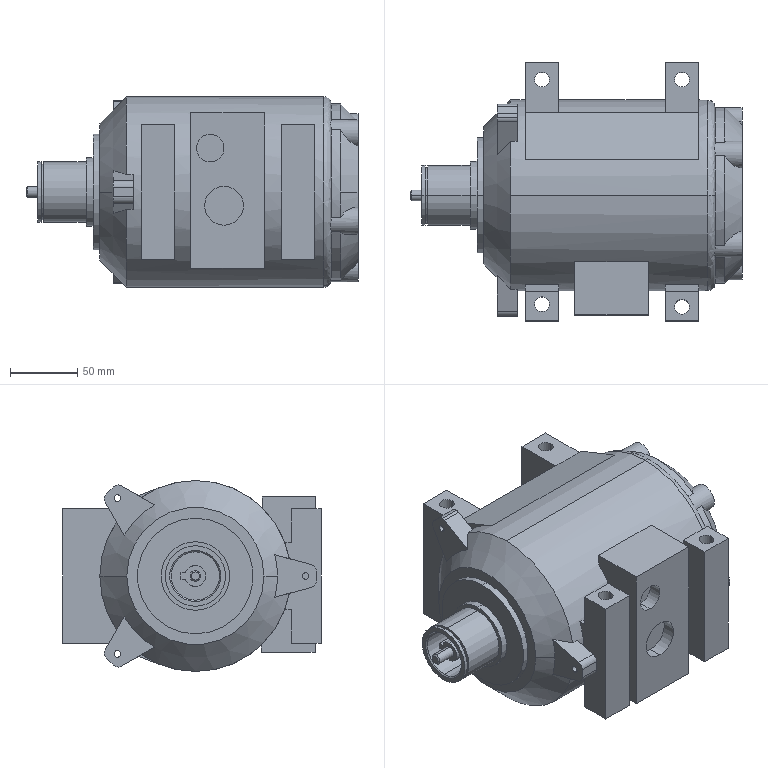Part | STEP file | PN_0001 cylinder body | 1 solid | 145 faces | box 246.9 x 192 x 142 mm | volume 3389900 mm3 | plane 72 | cylinder 59 | cone 12 | spline 2 | commonest cylinder face diameters 20 x10 11 x8 10 x7 5 x6 131 x5 45 x4